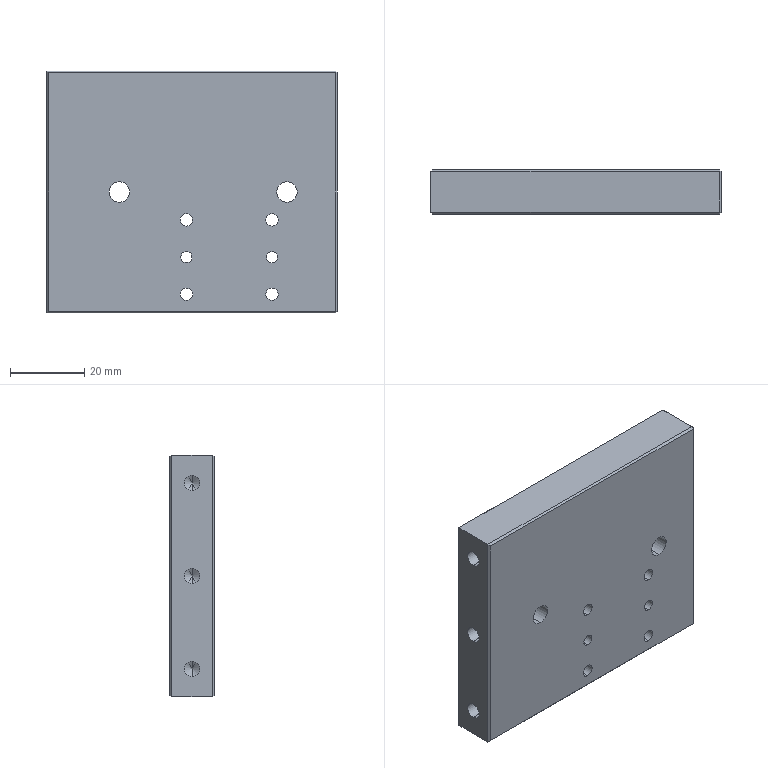Part | STEP file | ND25021-01-JDKM-60-TL | 1 solid | 54 faces | box 78 x 12 x 65 mm | volume 58491 mm3 | cylinder 26 | plane 22 | cone 6 | commonest cylinder face diameters 3.3 x8 4.2 x6 3 x4 5.5 x4 10 x4